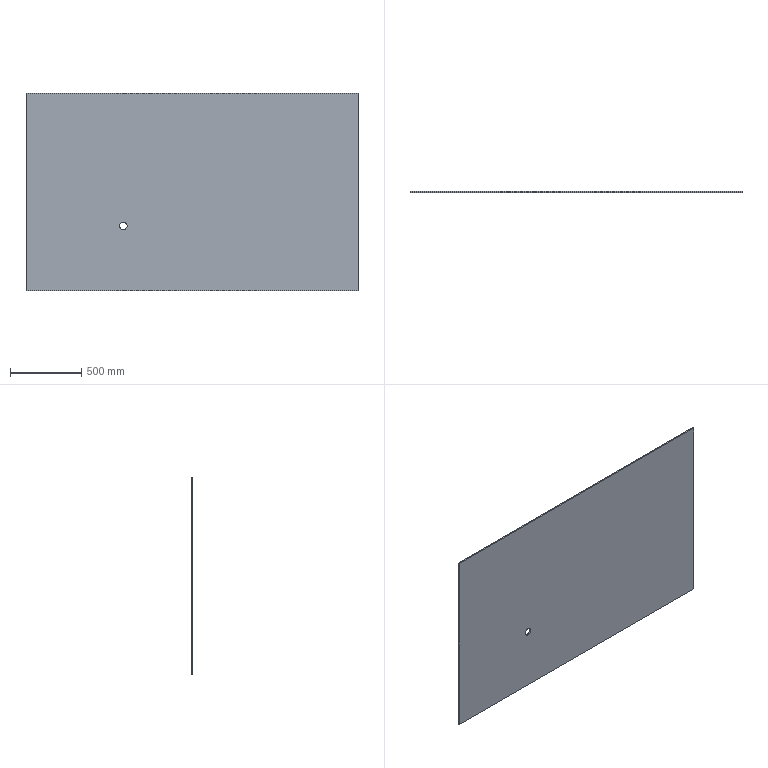Part | SolidWorks | features Extrusion 1 | 1 solid | 8 faces | box 2324 x 8 x 1380 mm | volume 25639970 mm3 | plane 6 | cylinder 2 | commonest cylinder face diameters 52 x2
STEP:
#1=CARTESIAN_POINT('',(-480.,4.,-263.));
#2=VERTEX_POINT('',#1);
#3=CARTESIAN_POINT('',(-480.,4.,-211.));
#4=VERTEX_POINT('',#3);
#5=CARTESIAN_POINT('',(-480.,4.,-237.));
#6=DIRECTION('',(0.,1.,0.));
#7=DIRECTION('',(0.,0.,1.));
#8=AXIS2_PLACEMENT_3D('',#5,#6,#7);
#9=CIRCLE('',#8,26.);
#10=EDGE_CURVE('',#2,#4,#9,.T.);
#11=ORIENTED_EDGE('',*,*,#10,.T.);
#12=CARTESIAN_POINT('',(-480.,-4.,-211.));
#13=VERTEX_POINT('',#12);
#14=CARTESIAN_POINT('',(-480.,4.,-211.));
#15=DIRECTION('',(0.,-1.,0.));
#16=VECTOR('',#15,1000.);
#17=LINE('',#14,#16);
#18=EDGE_CURVE('',#4,#13,#17,.T.);
#19=ORIENTED_EDGE('',*,*,#18,.T.);
#20=CARTESIAN_POINT('',(-480.,-4.,-263.));
#21=VERTEX_POINT('',#20);
#22=CARTESIAN_POINT('',(-480.,-4.,-237.));
#23=DIRECTION('',(0.,1.,0.));
#24=DIRECTION('',(0.,0.,1.));
#25=AXIS2_PLACEMENT_3D('',#22,#23,#24);
#26=CIRCLE('',#25,26.);
#27=EDGE_CURVE('',#21,#13,#26,.T.);
#28=ORIENTED_EDGE('',*,*,#27,.F.);
#29=CARTESIAN_POINT('',(-480.,4.,-263.));
#30=DIRECTION('',(0.,-1.,0.));
#31=VECTOR('',#30,1000.);
#32=LINE('',#29,#31);
#33=EDGE_CURVE('',#2,#21,#32,.T.);
#34=ORIENTED_EDGE('',*,*,#33,.F.);
#35=EDGE_LOOP('',(#11,#19,#28,#34));
#36=FACE_OUTER_BOUND('',#35,.T.);
#37=CARTESIAN_POINT('',(-480.,4.,-237.));
#38=DIRECTION('',(0.,-1.,0.));
#39=DIRECTION('',(0.,0.,-1.));
#40=AXIS2_PLACEMENT_3D('',#37,#38,#39);
#41=CYLINDRICAL_SURFACE('',#40,26.);
#42=ADVANCED_FACE('',(#36),#41,.F.);
#43=CARTESIAN_POINT('',(1162.,4.,690.));
#44=VERTEX_POINT('',#43);
#45=CARTESIAN_POINT('',(1162.,4.,-690.));
#46=VERTEX_POINT('',#45);
#47=CARTESIAN_POINT('',(1162.,4.,690.));
#48=DIRECTION('',(0.,0.,-1.));
#49=VECTOR('',#48,1000.);
#50=LINE('',#47,#49);
#51=EDGE_CURVE('',#44,#46,#50,.T.);
#52=ORIENTED_EDGE('',*,*,#51,.T.);
#53=CARTESIAN_POINT('',(-1162.,4.,-690.));
#54=VERTEX_POINT('',#53);
#55=CARTESIAN_POINT('',(-1162.,4.,-690.));
#56=DIRECTION('',(-1.,0.,0.));
#57=VECTOR('',#56,1000.);
#58=LINE('',#55,#57);
#59=EDGE_CURVE('',#46,#54,#58,.T.);
#60=ORIENTED_EDGE('',*,*,#59,.T.);
#61=CARTESIAN_POINT('',(-1162.,4.,690.));
#62=VERTEX_POINT('',#61);
#63=CARTESIAN_POINT('',(-1162.,4.,690.));
#64=DIRECTION('',(0.,0.,1.));
#65=VECTOR('',#64,1000.);
#66=LINE('',#63,#65);
#67=EDGE_CURVE('',#54,#62,#66,.T.);
#68=ORIENTED_EDGE('',*,*,#67,.T.);
#69=CARTESIAN_POINT('',(-1162.,4.,690.));
#70=DIRECTION('',(1.,0.,0.));
#71=VECTOR('',#70,1000.);
#72=LINE('',#69,#71);
#73=EDGE_CURVE('',#62,#44,#72,.T.);
#74=ORIENTED_EDGE('',*,*,#73,.T.);
#75=EDGE_LOOP('',(#52,#60,#68,#74));
#76=FACE_OUTER_BOUND('',#75,.T.);
#77=ORIENTED_EDGE('',*,*,#10,.F.);
#78=CARTESIAN_POINT('',(-480.,4.,-237.));
#79=DIRECTION('',(0.,1.,0.));
#80=DIRECTION('',(0.,0.,1.));
#81=AXIS2_PLACEMENT_3D('',#78,#79,#80);
#82=CIRCLE('',#81,26.);
#83=EDGE_CURVE('',#4,#2,#82,.T.);
#84=ORIENTED_EDGE('',*,*,#83,.F.);
#85=EDGE_LOOP('',(#77,#84));
#86=FACE_BOUND('',#85,.T.);
#87=CARTESIAN_POINT('',(0.,4.,0.));
#88=DIRECTION('',(0.,-1.,0.));
#89=DIRECTION('',(0.,0.,-1.));
#90=AXIS2_PLACEMENT_3D('',#87,#88,#89);
#91=PLANE('',#90);
#92=ADVANCED_FACE('',(#76,#86),#91,.F.);
#93=CARTESIAN_POINT('',(1162.,-4.,690.));
#94=VERTEX_POINT('',#93);
#95=CARTESIAN_POINT('',(1162.,-4.,-690.));
#96=VERTEX_POINT('',#95);
#97=CARTESIAN_POINT('',(1162.,-4.,690.));
#98=DIRECTION('',(0.,0.,-1.));
#99=VECTOR('',#98,1000.);
#100=LINE('',#97,#99);
#101=EDGE_CURVE('',#94,#96,#100,.T.);
#102=ORIENTED_EDGE('',*,*,#101,.F.);
#103=CARTESIAN_POINT('',(-1162.,-4.,690.));
#104=VERTEX_POINT('',#103);
#105=CARTESIAN_POINT('',(-1162.,-4.,690.));
#106=DIRECTION('',(1.,0.,0.));
#107=VECTOR('',#106,1000.);
#108=LINE('',#105,#107);
#109=EDGE_CURVE('',#104,#94,#108,.T.);
#110=ORIENTED_EDGE('',*,*,#109,.F.);
#111=CARTESIAN_POINT('',(-1162.,-4.,-690.));
#112=VERTEX_POINT('',#111);
#113=CARTESIAN_POINT('',(-1162.,-4.,690.));
#114=DIRECTION('',(0.,0.,1.));
#115=VECTOR('',#114,1000.);
#116=LINE('',#113,#115);
#117=EDGE_CURVE('',#112,#104,#116,.T.);
#118=ORIENTED_EDGE('',*,*,#117,.F.);
#119=CARTESIAN_POINT('',(-1162.,-4.,-690.));
#120=DIRECTION('',(-1.,0.,0.));
#121=VECTOR('',#120,1000.);
#122=LINE('',#119,#121);
#123=EDGE_CURVE('',#96,#112,#122,.T.);
#124=ORIENTED_EDGE('',*,*,#123,.F.);
#125=EDGE_LOOP('',(#102,#110,#118,#124));
#126=FACE_OUTER_BOUND('',#125,.T.);
#127=ORIENTED_EDGE('',*,*,#27,.T.);
#128=CARTESIAN_POINT('',(-480.,-4.,-237.));
#129=DIRECTION('',(0.,1.,0.));
#130=DIRECTION('',(0.,0.,1.));
#131=AXIS2_PLACEMENT_3D('',#128,#129,#130);
#132=CIRCLE('',#131,26.);
#133=EDGE_CURVE('',#13,#21,#132,.T.);
#134=ORIENTED_EDGE('',*,*,#133,.T.);
#135=EDGE_LOOP('',(#127,#134));
#136=FACE_BOUND('',#135,.T.);
#137=CARTESIAN_POINT('',(0.,-4.,0.));
#138=DIRECTION('',(0.,-1.,0.));
#139=DIRECTION('',(0.,0.,-1.));
#140=AXIS2_PLACEMENT_3D('',#137,#138,#139);
#141=PLANE('',#140);
#142=ADVANCED_FACE('',(#126,#136),#141,.T.);
#143=ORIENTED_EDGE('',*,*,#101,.T.);
#144=CARTESIAN_POINT('',(1162.,4.,-690.));
#145=DIRECTION('',(0.,-1.,0.));
#146=VECTOR('',#145,1000.);
#147=LINE('',#144,#146);
#148=EDGE_CURVE('',#46,#96,#147,.T.);
#149=ORIENTED_EDGE('',*,*,#148,.F.);
#150=ORIENTED_EDGE('',*,*,#51,.F.);
#151=CARTESIAN_POINT('',(1162.,4.,690.));
#152=DIRECTION('',(0.,-1.,0.));
#153=VECTOR('',#152,1000.);
#154=LINE('',#151,#153);
#155=EDGE_CURVE('',#44,#94,#154,.T.);
#156=ORIENTED_EDGE('',*,*,#155,.T.);
#157=EDGE_LOOP('',(#143,#149,#150,#156));
#158=FACE_OUTER_BOUND('',#157,.T.);
#159=CARTESIAN_POINT('',(1162.,4.,690.));
#160=DIRECTION('',(-1.,0.,0.));
#161=DIRECTION('',(0.,0.,1.));
#162=AXIS2_PLACEMENT_3D('',#159,#160,#161);
#163=PLANE('',#162);
#164=ADVANCED_FACE('',(#158),#163,.F.);
#165=ORIENTED_EDGE('',*,*,#123,.T.);
#166=CARTESIAN_POINT('',(-1162.,4.,-690.));
#167=DIRECTION('',(0.,-1.,0.));
#168=VECTOR('',#167,1000.);
#169=LINE('',#166,#168);
#170=EDGE_CURVE('',#54,#112,#169,.T.);
#171=ORIENTED_EDGE('',*,*,#170,.F.);
#172=ORIENTED_EDGE('',*,*,#59,.F.);
#173=ORIENTED_EDGE('',*,*,#148,.T.);
#174=EDGE_LOOP('',(#165,#171,#172,#173));
#175=FACE_OUTER_BOUND('',#174,.T.);
#176=CARTESIAN_POINT('',(-1162.,4.,-690.));
#177=DIRECTION('',(0.,0.,1.));
#178=DIRECTION('',(1.,0.,0.));
#179=AXIS2_PLACEMENT_3D('',#176,#177,#178);
#180=PLANE('',#179);
#181=ADVANCED_FACE('',(#175),#180,.F.);
#182=ORIENTED_EDGE('',*,*,#117,.T.);
#183=CARTESIAN_POINT('',(-1162.,4.,690.));
#184=DIRECTION('',(0.,-1.,0.));
#185=VECTOR('',#184,1000.);
#186=LINE('',#183,#185);
#187=EDGE_CURVE('',#62,#104,#186,.T.);
#188=ORIENTED_EDGE('',*,*,#187,.F.);
#189=ORIENTED_EDGE('',*,*,#67,.F.);
#190=ORIENTED_EDGE('',*,*,#170,.T.);
#191=EDGE_LOOP('',(#182,#188,#189,#190));
#192=FACE_OUTER_BOUND('',#191,.T.);
#193=CARTESIAN_POINT('',(-1162.,4.,690.));
#194=DIRECTION('',(1.,0.,0.));
#195=DIRECTION('',(0.,0.,-1.));
#196=AXIS2_PLACEMENT_3D('',#193,#194,#195);
#197=PLANE('',#196);
#198=ADVANCED_FACE('',(#192),#197,.F.);
#199=ORIENTED_EDGE('',*,*,#109,.T.);
#200=ORIENTED_EDGE('',*,*,#155,.F.);
#201=ORIENTED_EDGE('',*,*,#73,.F.);
#202=ORIENTED_EDGE('',*,*,#187,.T.);
#203=EDGE_LOOP('',(#199,#200,#201,#202));
#204=FACE_OUTER_BOUND('',#203,.T.);
#205=CARTESIAN_POINT('',(-1162.,4.,690.));
#206=DIRECTION('',(0.,0.,-1.));
#207=DIRECTION('',(-1.,0.,0.));
#208=AXIS2_PLACEMENT_3D('',#205,#206,#207);
#209=PLANE('',#208);
#210=ADVANCED_FACE('',(#204),#209,.F.);
#211=ORIENTED_EDGE('',*,*,#18,.F.);
#212=ORIENTED_EDGE('',*,*,#83,.T.);
#213=ORIENTED_EDGE('',*,*,#33,.T.);
#214=ORIENTED_EDGE('',*,*,#133,.F.);
#215=EDGE_LOOP('',(#211,#212,#213,#214));
#216=FACE_OUTER_BOUND('',#215,.T.);
#217=CARTESIAN_POINT('',(-480.,4.,-237.));
#218=DIRECTION('',(0.,-1.,0.));
#219=DIRECTION('',(0.,0.,-1.));
#220=AXIS2_PLACEMENT_3D('',#217,#218,#219);
#221=CYLINDRICAL_SURFACE('',#220,26.);
#222=ADVANCED_FACE('',(#216),#221,.F.);
#223=CLOSED_SHELL('',(#42,#92,#142,#164,#181,#198,#210,#222));
#224=MANIFOLD_SOLID_BREP('',#223);
#225=CARTESIAN_POINT('',(0.,0.,0.));
#226=DIRECTION('',(0.,0.,1.));
#227=DIRECTION('',(1.,0.,0.));
#228=AXIS2_PLACEMENT_3D('',#225,#226,#227);
#229=(LENGTH_UNIT()NAMED_UNIT(*)SI_UNIT(.MILLI.,.METRE.));
#230=UNCERTAINTY_MEASURE_WITH_UNIT(LENGTH_MEASURE(0.00001),#229,'','');
#231=(NAMED_UNIT(*)PLANE_ANGLE_UNIT()SI_UNIT($,.RADIAN.));
#232=(NAMED_UNIT(*)SI_UNIT($,.STERADIAN.)SOLID_ANGLE_UNIT());
#233=(GEOMETRIC_REPRESENTATION_CONTEXT(3)GLOBAL_UNCERTAINTY_ASSIGNED_CONTEXT((#230))GLOBAL_UNIT_ASSIGNED_CONTEXT((#229,#231,#232))REPRESENTATION_CONTEXT('',''));
#234=ADVANCED_BREP_SHAPE_REPRESENTATION('',(#224,#228),#233);